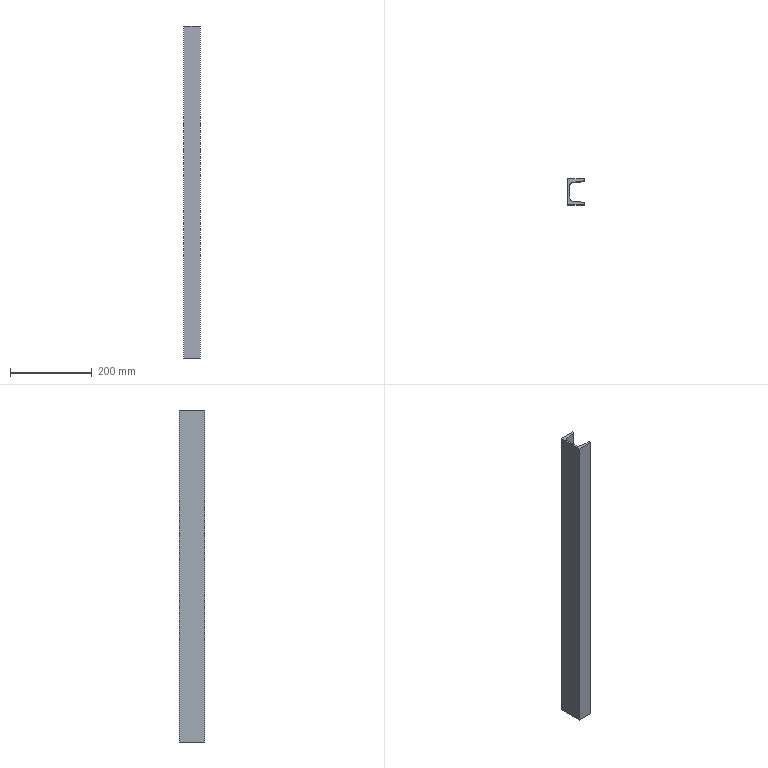Part | STEP file | 750038457 | 1 solid | 14 faces | box 40 x 63 x 810 mm | volume 684099 mm3 | plane 10 | cylinder 4 | commonest cylinder face diameters 7.6 x2 15 x2
STEP:
#1=CARTESIAN_POINT('',(0.,0.,810.));
#2=VERTEX_POINT('',#1);
#3=CARTESIAN_POINT('',(0.,0.,0.));
#4=VERTEX_POINT('',#3);
#5=CARTESIAN_POINT('',(0.,0.,810.));
#6=DIRECTION('',(0.,0.,-1.));
#7=VECTOR('',#6,1000.);
#8=LINE('',#5,#7);
#9=EDGE_CURVE('',#2,#4,#8,.T.);
#10=ORIENTED_EDGE('',*,*,#9,.F.);
#11=CARTESIAN_POINT('',(0.,63.,810.));
#12=VERTEX_POINT('',#11);
#13=CARTESIAN_POINT('',(0.,63.,810.));
#14=DIRECTION('',(0.,-1.,0.));
#15=VECTOR('',#14,1000.);
#16=LINE('',#13,#15);
#17=EDGE_CURVE('',#12,#2,#16,.T.);
#18=ORIENTED_EDGE('',*,*,#17,.F.);
#19=CARTESIAN_POINT('',(0.,63.,0.));
#20=VERTEX_POINT('',#19);
#21=CARTESIAN_POINT('',(0.,63.,810.));
#22=DIRECTION('',(0.,0.,1.));
#23=VECTOR('',#22,1000.);
#24=LINE('',#21,#23);
#25=EDGE_CURVE('',#20,#12,#24,.T.);
#26=ORIENTED_EDGE('',*,*,#25,.F.);
#27=CARTESIAN_POINT('',(0.,63.,0.));
#28=DIRECTION('',(0.,1.,0.));
#29=VECTOR('',#28,1000.);
#30=LINE('',#27,#29);
#31=EDGE_CURVE('',#4,#20,#30,.T.);
#32=ORIENTED_EDGE('',*,*,#31,.F.);
#33=EDGE_LOOP('',(#10,#18,#26,#32));
#34=FACE_OUTER_BOUND('',#33,.T.);
#35=CARTESIAN_POINT('',(0.,63.,810.));
#36=DIRECTION('',(1.,0.,0.));
#37=DIRECTION('',(0.,0.,-1.));
#38=AXIS2_PLACEMENT_3D('',#35,#36,#37);
#39=PLANE('',#38);
#40=ADVANCED_FACE('',(#34),#39,.F.);
#41=CARTESIAN_POINT('',(40.,63.,0.));
#42=VERTEX_POINT('',#41);
#43=CARTESIAN_POINT('',(36.2,63.,0.));
#44=DIRECTION('',(-1.,0.,0.));
#45=VECTOR('',#44,1000.);
#46=LINE('',#43,#45);
#47=EDGE_CURVE('',#42,#20,#46,.T.);
#48=ORIENTED_EDGE('',*,*,#47,.F.);
#49=CARTESIAN_POINT('',(40.,60.699,0.));
#50=VERTEX_POINT('',#49);
#51=CARTESIAN_POINT('',(40.,2.301,0.));
#52=DIRECTION('',(0.,1.,0.));
#53=VECTOR('',#52,1000.);
#54=LINE('',#51,#53);
#55=EDGE_CURVE('',#50,#42,#54,.T.);
#56=ORIENTED_EDGE('',*,*,#55,.F.);
#57=CARTESIAN_POINT('',(36.578,56.918,0.));
#58=VERTEX_POINT('',#57);
#59=CARTESIAN_POINT('',(36.2,60.699,0.));
#60=DIRECTION('',(0.,0.,1.));
#61=DIRECTION('',(-1.,0.,0.));
#62=AXIS2_PLACEMENT_3D('',#59,#60,#61);
#63=CIRCLE('',#62,3.8);
#64=EDGE_CURVE('',#58,#50,#63,.T.);
#65=ORIENTED_EDGE('',*,*,#64,.F.);
#66=CARTESIAN_POINT('',(11.554,54.415,0.));
#67=VERTEX_POINT('',#66);
#68=CARTESIAN_POINT('',(11.554,54.415,0.));
#69=DIRECTION('',(0.995,0.0995,0.));
#70=VECTOR('',#69,1000.);
#71=LINE('',#68,#70);
#72=EDGE_CURVE('',#67,#58,#71,.T.);
#73=ORIENTED_EDGE('',*,*,#72,.F.);
#74=CARTESIAN_POINT('',(4.8,46.953,0.));
#75=VERTEX_POINT('',#74);
#76=CARTESIAN_POINT('',(12.3,46.953,0.));
#77=DIRECTION('',(0.,0.,-1.));
#78=DIRECTION('',(-1.,0.,0.));
#79=AXIS2_PLACEMENT_3D('',#76,#77,#78);
#80=CIRCLE('',#79,7.5);
#81=EDGE_CURVE('',#75,#67,#80,.T.);
#82=ORIENTED_EDGE('',*,*,#81,.F.);
#83=CARTESIAN_POINT('',(4.8,16.047,0.));
#84=VERTEX_POINT('',#83);
#85=CARTESIAN_POINT('',(4.8,2.301,0.));
#86=DIRECTION('',(0.,1.,0.));
#87=VECTOR('',#86,1000.);
#88=LINE('',#85,#87);
#89=EDGE_CURVE('',#84,#75,#88,.T.);
#90=ORIENTED_EDGE('',*,*,#89,.F.);
#91=CARTESIAN_POINT('',(11.554,8.585,0.));
#92=VERTEX_POINT('',#91);
#93=CARTESIAN_POINT('',(12.3,16.047,0.));
#94=DIRECTION('',(0.,0.,-1.));
#95=DIRECTION('',(-1.,0.,0.));
#96=AXIS2_PLACEMENT_3D('',#93,#94,#95);
#97=CIRCLE('',#96,7.5);
#98=EDGE_CURVE('',#92,#84,#97,.T.);
#99=ORIENTED_EDGE('',*,*,#98,.F.);
#100=CARTESIAN_POINT('',(36.578,6.082,0.));
#101=VERTEX_POINT('',#100);
#102=CARTESIAN_POINT('',(36.578,6.082,0.));
#103=DIRECTION('',(-0.995,0.0995,0.));
#104=VECTOR('',#103,1000.);
#105=LINE('',#102,#104);
#106=EDGE_CURVE('',#101,#92,#105,.T.);
#107=ORIENTED_EDGE('',*,*,#106,.F.);
#108=CARTESIAN_POINT('',(40.,2.301,0.));
#109=VERTEX_POINT('',#108);
#110=CARTESIAN_POINT('',(36.2,2.301,0.));
#111=DIRECTION('',(0.,0.,1.));
#112=DIRECTION('',(-1.,0.,0.));
#113=AXIS2_PLACEMENT_3D('',#110,#111,#112);
#114=CIRCLE('',#113,3.8);
#115=EDGE_CURVE('',#109,#101,#114,.T.);
#116=ORIENTED_EDGE('',*,*,#115,.F.);
#117=CARTESIAN_POINT('',(40.,0.,0.));
#118=VERTEX_POINT('',#117);
#119=CARTESIAN_POINT('',(40.,2.301,0.));
#120=DIRECTION('',(0.,1.,0.));
#121=VECTOR('',#120,1000.);
#122=LINE('',#119,#121);
#123=EDGE_CURVE('',#118,#109,#122,.T.);
#124=ORIENTED_EDGE('',*,*,#123,.F.);
#125=CARTESIAN_POINT('',(36.2,0.,0.));
#126=DIRECTION('',(1.,0.,0.));
#127=VECTOR('',#126,1000.);
#128=LINE('',#125,#127);
#129=EDGE_CURVE('',#4,#118,#128,.T.);
#130=ORIENTED_EDGE('',*,*,#129,.F.);
#131=ORIENTED_EDGE('',*,*,#31,.T.);
#132=EDGE_LOOP('',(#48,#56,#65,#73,#82,#90,#99,#107,#116,#124,#130,#131));
#133=FACE_OUTER_BOUND('',#132,.T.);
#134=CARTESIAN_POINT('',(36.2,2.301,0.));
#135=DIRECTION('',(0.,0.,1.));
#136=DIRECTION('',(1.,0.,0.));
#137=AXIS2_PLACEMENT_3D('',#134,#135,#136);
#138=PLANE('',#137);
#139=ADVANCED_FACE('',(#133),#138,.F.);
#140=CARTESIAN_POINT('',(40.,0.,810.));
#141=VERTEX_POINT('',#140);
#142=CARTESIAN_POINT('',(40.,0.,810.));
#143=DIRECTION('',(0.,0.,-1.));
#144=VECTOR('',#143,1000.);
#145=LINE('',#142,#144);
#146=EDGE_CURVE('',#141,#118,#145,.T.);
#147=ORIENTED_EDGE('',*,*,#146,.F.);
#148=CARTESIAN_POINT('',(0.,0.,810.));
#149=DIRECTION('',(1.,0.,0.));
#150=VECTOR('',#149,1000.);
#151=LINE('',#148,#150);
#152=EDGE_CURVE('',#2,#141,#151,.T.);
#153=ORIENTED_EDGE('',*,*,#152,.F.);
#154=ORIENTED_EDGE('',*,*,#9,.T.);
#155=ORIENTED_EDGE('',*,*,#129,.T.);
#156=EDGE_LOOP('',(#147,#153,#154,#155));
#157=FACE_OUTER_BOUND('',#156,.T.);
#158=CARTESIAN_POINT('',(0.,0.,810.));
#159=DIRECTION('',(0.,1.,0.));
#160=DIRECTION('',(0.,0.,1.));
#161=AXIS2_PLACEMENT_3D('',#158,#159,#160);
#162=PLANE('',#161);
#163=ADVANCED_FACE('',(#157),#162,.F.);
#164=CARTESIAN_POINT('',(40.,60.699,810.));
#165=VERTEX_POINT('',#164);
#166=CARTESIAN_POINT('',(40.,63.,810.));
#167=VERTEX_POINT('',#166);
#168=CARTESIAN_POINT('',(40.,2.301,810.));
#169=DIRECTION('',(0.,1.,0.));
#170=VECTOR('',#169,1000.);
#171=LINE('',#168,#170);
#172=EDGE_CURVE('',#165,#167,#171,.T.);
#173=ORIENTED_EDGE('',*,*,#172,.T.);
#174=CARTESIAN_POINT('',(36.2,63.,810.));
#175=DIRECTION('',(-1.,0.,0.));
#176=VECTOR('',#175,1000.);
#177=LINE('',#174,#176);
#178=EDGE_CURVE('',#167,#12,#177,.T.);
#179=ORIENTED_EDGE('',*,*,#178,.T.);
#180=ORIENTED_EDGE('',*,*,#17,.T.);
#181=ORIENTED_EDGE('',*,*,#152,.T.);
#182=CARTESIAN_POINT('',(40.,2.301,810.));
#183=VERTEX_POINT('',#182);
#184=CARTESIAN_POINT('',(40.,2.301,810.));
#185=DIRECTION('',(0.,1.,0.));
#186=VECTOR('',#185,1000.);
#187=LINE('',#184,#186);
#188=EDGE_CURVE('',#141,#183,#187,.T.);
#189=ORIENTED_EDGE('',*,*,#188,.T.);
#190=CARTESIAN_POINT('',(36.578,6.082,810.));
#191=VERTEX_POINT('',#190);
#192=CARTESIAN_POINT('',(36.2,2.301,810.));
#193=DIRECTION('',(0.,0.,1.));
#194=DIRECTION('',(-1.,0.,0.));
#195=AXIS2_PLACEMENT_3D('',#192,#193,#194);
#196=CIRCLE('',#195,3.8);
#197=EDGE_CURVE('',#183,#191,#196,.T.);
#198=ORIENTED_EDGE('',*,*,#197,.T.);
#199=CARTESIAN_POINT('',(11.554,8.585,810.));
#200=VERTEX_POINT('',#199);
#201=CARTESIAN_POINT('',(36.578,6.082,810.));
#202=DIRECTION('',(-0.995,0.0995,0.));
#203=VECTOR('',#202,1000.);
#204=LINE('',#201,#203);
#205=EDGE_CURVE('',#191,#200,#204,.T.);
#206=ORIENTED_EDGE('',*,*,#205,.T.);
#207=CARTESIAN_POINT('',(4.8,16.047,810.));
#208=VERTEX_POINT('',#207);
#209=CARTESIAN_POINT('',(12.3,16.047,810.));
#210=DIRECTION('',(0.,0.,-1.));
#211=DIRECTION('',(-1.,0.,0.));
#212=AXIS2_PLACEMENT_3D('',#209,#210,#211);
#213=CIRCLE('',#212,7.5);
#214=EDGE_CURVE('',#200,#208,#213,.T.);
#215=ORIENTED_EDGE('',*,*,#214,.T.);
#216=CARTESIAN_POINT('',(4.8,46.953,810.));
#217=VERTEX_POINT('',#216);
#218=CARTESIAN_POINT('',(4.8,2.301,810.));
#219=DIRECTION('',(0.,1.,0.));
#220=VECTOR('',#219,1000.);
#221=LINE('',#218,#220);
#222=EDGE_CURVE('',#208,#217,#221,.T.);
#223=ORIENTED_EDGE('',*,*,#222,.T.);
#224=CARTESIAN_POINT('',(11.554,54.415,810.));
#225=VERTEX_POINT('',#224);
#226=CARTESIAN_POINT('',(12.3,46.953,810.));
#227=DIRECTION('',(0.,0.,-1.));
#228=DIRECTION('',(-1.,0.,0.));
#229=AXIS2_PLACEMENT_3D('',#226,#227,#228);
#230=CIRCLE('',#229,7.5);
#231=EDGE_CURVE('',#217,#225,#230,.T.);
#232=ORIENTED_EDGE('',*,*,#231,.T.);
#233=CARTESIAN_POINT('',(36.578,56.918,810.));
#234=VERTEX_POINT('',#233);
#235=CARTESIAN_POINT('',(11.554,54.415,810.));
#236=DIRECTION('',(0.995,0.0995,0.));
#237=VECTOR('',#236,1000.);
#238=LINE('',#235,#237);
#239=EDGE_CURVE('',#225,#234,#238,.T.);
#240=ORIENTED_EDGE('',*,*,#239,.T.);
#241=CARTESIAN_POINT('',(36.2,60.699,810.));
#242=DIRECTION('',(0.,0.,1.));
#243=DIRECTION('',(-1.,0.,0.));
#244=AXIS2_PLACEMENT_3D('',#241,#242,#243);
#245=CIRCLE('',#244,3.8);
#246=EDGE_CURVE('',#234,#165,#245,.T.);
#247=ORIENTED_EDGE('',*,*,#246,.T.);
#248=EDGE_LOOP('',(#173,#179,#180,#181,#189,#198,#206,#215,#223,#232,#240,#247));
#249=FACE_OUTER_BOUND('',#248,.T.);
#250=CARTESIAN_POINT('',(36.2,2.301,810.));
#251=DIRECTION('',(0.,0.,1.));
#252=DIRECTION('',(1.,0.,0.));
#253=AXIS2_PLACEMENT_3D('',#250,#251,#252);
#254=PLANE('',#253);
#255=ADVANCED_FACE('',(#249),#254,.T.);
#256=ORIENTED_EDGE('',*,*,#25,.T.);
#257=ORIENTED_EDGE('',*,*,#178,.F.);
#258=CARTESIAN_POINT('',(40.,63.,810.));
#259=DIRECTION('',(0.,0.,1.));
#260=VECTOR('',#259,1000.);
#261=LINE('',#258,#260);
#262=EDGE_CURVE('',#42,#167,#261,.T.);
#263=ORIENTED_EDGE('',*,*,#262,.F.);
#264=ORIENTED_EDGE('',*,*,#47,.T.);
#265=EDGE_LOOP('',(#256,#257,#263,#264));
#266=FACE_OUTER_BOUND('',#265,.T.);
#267=CARTESIAN_POINT('',(40.,63.,810.));
#268=DIRECTION('',(0.,-1.,0.));
#269=DIRECTION('',(0.,0.,-1.));
#270=AXIS2_PLACEMENT_3D('',#267,#268,#269);
#271=PLANE('',#270);
#272=ADVANCED_FACE('',(#266),#271,.F.);
#273=ORIENTED_EDGE('',*,*,#262,.T.);
#274=ORIENTED_EDGE('',*,*,#172,.F.);
#275=CARTESIAN_POINT('',(40.,60.699,810.));
#276=DIRECTION('',(0.,0.,1.));
#277=VECTOR('',#276,1000.);
#278=LINE('',#275,#277);
#279=EDGE_CURVE('',#50,#165,#278,.T.);
#280=ORIENTED_EDGE('',*,*,#279,.F.);
#281=ORIENTED_EDGE('',*,*,#55,.T.);
#282=EDGE_LOOP('',(#273,#274,#280,#281));
#283=FACE_OUTER_BOUND('',#282,.T.);
#284=CARTESIAN_POINT('',(40.,60.699,810.));
#285=DIRECTION('',(-1.,0.,0.));
#286=DIRECTION('',(0.,-1.,0.));
#287=AXIS2_PLACEMENT_3D('',#284,#285,#286);
#288=PLANE('',#287);
#289=ADVANCED_FACE('',(#283),#288,.F.);
#290=ORIENTED_EDGE('',*,*,#246,.F.);
#291=CARTESIAN_POINT('',(36.578,56.918,810.));
#292=DIRECTION('',(0.,0.,-1.));
#293=VECTOR('',#292,1000.);
#294=LINE('',#291,#293);
#295=EDGE_CURVE('',#234,#58,#294,.T.);
#296=ORIENTED_EDGE('',*,*,#295,.T.);
#297=ORIENTED_EDGE('',*,*,#64,.T.);
#298=ORIENTED_EDGE('',*,*,#279,.T.);
#299=EDGE_LOOP('',(#290,#296,#297,#298));
#300=FACE_OUTER_BOUND('',#299,.T.);
#301=CARTESIAN_POINT('',(36.2,60.699,810.));
#302=DIRECTION('',(0.,0.,-1.));
#303=DIRECTION('',(-1.,0.,0.));
#304=AXIS2_PLACEMENT_3D('',#301,#302,#303);
#305=CYLINDRICAL_SURFACE('',#304,3.8);
#306=ADVANCED_FACE('',(#300),#305,.T.);
#307=ORIENTED_EDGE('',*,*,#295,.F.);
#308=ORIENTED_EDGE('',*,*,#239,.F.);
#309=CARTESIAN_POINT('',(11.554,54.415,810.));
#310=DIRECTION('',(0.,0.,1.));
#311=VECTOR('',#310,1000.);
#312=LINE('',#309,#311);
#313=EDGE_CURVE('',#67,#225,#312,.T.);
#314=ORIENTED_EDGE('',*,*,#313,.F.);
#315=ORIENTED_EDGE('',*,*,#72,.T.);
#316=EDGE_LOOP('',(#307,#308,#314,#315));
#317=FACE_OUTER_BOUND('',#316,.T.);
#318=CARTESIAN_POINT('',(11.554,54.415,810.));
#319=DIRECTION('',(-0.0995,0.995,0.));
#320=DIRECTION('',(-0.995,-0.0995,0.));
#321=AXIS2_PLACEMENT_3D('',#318,#319,#320);
#322=PLANE('',#321);
#323=ADVANCED_FACE('',(#317),#322,.F.);
#324=ORIENTED_EDGE('',*,*,#313,.T.);
#325=ORIENTED_EDGE('',*,*,#231,.F.);
#326=CARTESIAN_POINT('',(4.8,46.953,810.));
#327=DIRECTION('',(0.,0.,1.));
#328=VECTOR('',#327,1000.);
#329=LINE('',#326,#328);
#330=EDGE_CURVE('',#75,#217,#329,.T.);
#331=ORIENTED_EDGE('',*,*,#330,.F.);
#332=ORIENTED_EDGE('',*,*,#81,.T.);
#333=EDGE_LOOP('',(#324,#325,#331,#332));
#334=FACE_OUTER_BOUND('',#333,.T.);
#335=CARTESIAN_POINT('',(12.3,46.953,810.));
#336=DIRECTION('',(0.,0.,-1.));
#337=DIRECTION('',(-1.,0.,0.));
#338=AXIS2_PLACEMENT_3D('',#335,#336,#337);
#339=CYLINDRICAL_SURFACE('',#338,7.5);
#340=ADVANCED_FACE('',(#334),#339,.F.);
#341=ORIENTED_EDGE('',*,*,#330,.T.);
#342=ORIENTED_EDGE('',*,*,#222,.F.);
#343=CARTESIAN_POINT('',(4.8,16.047,810.));
#344=DIRECTION('',(0.,0.,1.));
#345=VECTOR('',#344,1000.);
#346=LINE('',#343,#345);
#347=EDGE_CURVE('',#84,#208,#346,.T.);
#348=ORIENTED_EDGE('',*,*,#347,.F.);
#349=ORIENTED_EDGE('',*,*,#89,.T.);
#350=EDGE_LOOP('',(#341,#342,#348,#349));
#351=FACE_OUTER_BOUND('',#350,.T.);
#352=CARTESIAN_POINT('',(4.8,16.047,810.));
#353=DIRECTION('',(-1.,0.,0.));
#354=DIRECTION('',(0.,-1.,0.));
#355=AXIS2_PLACEMENT_3D('',#352,#353,#354);
#356=PLANE('',#355);
#357=ADVANCED_FACE('',(#351),#356,.F.);
#358=ORIENTED_EDGE('',*,*,#347,.T.);
#359=ORIENTED_EDGE('',*,*,#214,.F.);
#360=CARTESIAN_POINT('',(11.554,8.585,810.));
#361=DIRECTION('',(0.,0.,1.));
#362=VECTOR('',#361,1000.);
#363=LINE('',#360,#362);
#364=EDGE_CURVE('',#92,#200,#363,.T.);
#365=ORIENTED_EDGE('',*,*,#364,.F.);
#366=ORIENTED_EDGE('',*,*,#98,.T.);
#367=EDGE_LOOP('',(#358,#359,#365,#366));
#368=FACE_OUTER_BOUND('',#367,.T.);
#369=CARTESIAN_POINT('',(12.3,16.047,810.));
#370=DIRECTION('',(0.,0.,-1.));
#371=DIRECTION('',(-1.,0.,0.));
#372=AXIS2_PLACEMENT_3D('',#369,#370,#371);
#373=CYLINDRICAL_SURFACE('',#372,7.5);
#374=ADVANCED_FACE('',(#368),#373,.F.);
#375=ORIENTED_EDGE('',*,*,#364,.T.);
#376=ORIENTED_EDGE('',*,*,#205,.F.);
#377=CARTESIAN_POINT('',(36.578,6.082,810.));
#378=DIRECTION('',(0.,0.,1.));
#379=VECTOR('',#378,1000.);
#380=LINE('',#377,#379);
#381=EDGE_CURVE('',#101,#191,#380,.T.);
#382=ORIENTED_EDGE('',*,*,#381,.F.);
#383=ORIENTED_EDGE('',*,*,#106,.T.);
#384=EDGE_LOOP('',(#375,#376,#382,#383));
#385=FACE_OUTER_BOUND('',#384,.T.);
#386=CARTESIAN_POINT('',(36.578,6.082,810.));
#387=DIRECTION('',(-0.0995,-0.995,0.));
#388=DIRECTION('',(0.995,-0.0995,0.));
#389=AXIS2_PLACEMENT_3D('',#386,#387,#388);
#390=PLANE('',#389);
#391=ADVANCED_FACE('',(#385),#390,.F.);
#392=ORIENTED_EDGE('',*,*,#197,.F.);
#393=CARTESIAN_POINT('',(40.,2.301,810.));
#394=DIRECTION('',(0.,0.,-1.));
#395=VECTOR('',#394,1000.);
#396=LINE('',#393,#395);
#397=EDGE_CURVE('',#183,#109,#396,.T.);
#398=ORIENTED_EDGE('',*,*,#397,.T.);
#399=ORIENTED_EDGE('',*,*,#115,.T.);
#400=ORIENTED_EDGE('',*,*,#381,.T.);
#401=EDGE_LOOP('',(#392,#398,#399,#400));
#402=FACE_OUTER_BOUND('',#401,.T.);
#403=CARTESIAN_POINT('',(36.2,2.301,810.));
#404=DIRECTION('',(0.,0.,-1.));
#405=DIRECTION('',(-1.,0.,0.));
#406=AXIS2_PLACEMENT_3D('',#403,#404,#405);
#407=CYLINDRICAL_SURFACE('',#406,3.8);
#408=ADVANCED_FACE('',(#402),#407,.T.);
#409=ORIENTED_EDGE('',*,*,#397,.F.);
#410=ORIENTED_EDGE('',*,*,#188,.F.);
#411=ORIENTED_EDGE('',*,*,#146,.T.);
#412=ORIENTED_EDGE('',*,*,#123,.T.);
#413=EDGE_LOOP('',(#409,#410,#411,#412));
#414=FACE_OUTER_BOUND('',#413,.T.);
#415=CARTESIAN_POINT('',(40.,0.,810.));
#416=DIRECTION('',(-1.,0.,0.));
#417=DIRECTION('',(0.,0.,1.));
#418=AXIS2_PLACEMENT_3D('',#415,#416,#417);
#419=PLANE('',#418);
#420=ADVANCED_FACE('',(#414),#419,.F.);
#421=CLOSED_SHELL('',(#40,#139,#163,#255,#272,#289,#306,#323,#340,#357,#374,#391,#408,#420));
#422=MANIFOLD_SOLID_BREP('',#421);
#423=CARTESIAN_POINT('',(0.,0.,0.));
#424=DIRECTION('',(0.,0.,1.));
#425=DIRECTION('',(1.,0.,0.));
#426=AXIS2_PLACEMENT_3D('',#423,#424,#425);
#427=(LENGTH_UNIT()NAMED_UNIT(*)SI_UNIT(.MILLI.,.METRE.));
#428=UNCERTAINTY_MEASURE_WITH_UNIT(LENGTH_MEASURE(0.00001),#427,'','');
#429=(NAMED_UNIT(*)PLANE_ANGLE_UNIT()SI_UNIT($,.RADIAN.));
#430=(NAMED_UNIT(*)SI_UNIT($,.STERADIAN.)SOLID_ANGLE_UNIT());
#431=(GEOMETRIC_REPRESENTATION_CONTEXT(3)GLOBAL_UNCERTAINTY_ASSIGNED_CONTEXT((#428))GLOBAL_UNIT_ASSIGNED_CONTEXT((#427,#429,#430))REPRESENTATION_CONTEXT('',''));
#432=ADVANCED_BREP_SHAPE_REPRESENTATION('',(#422,#426),#431);